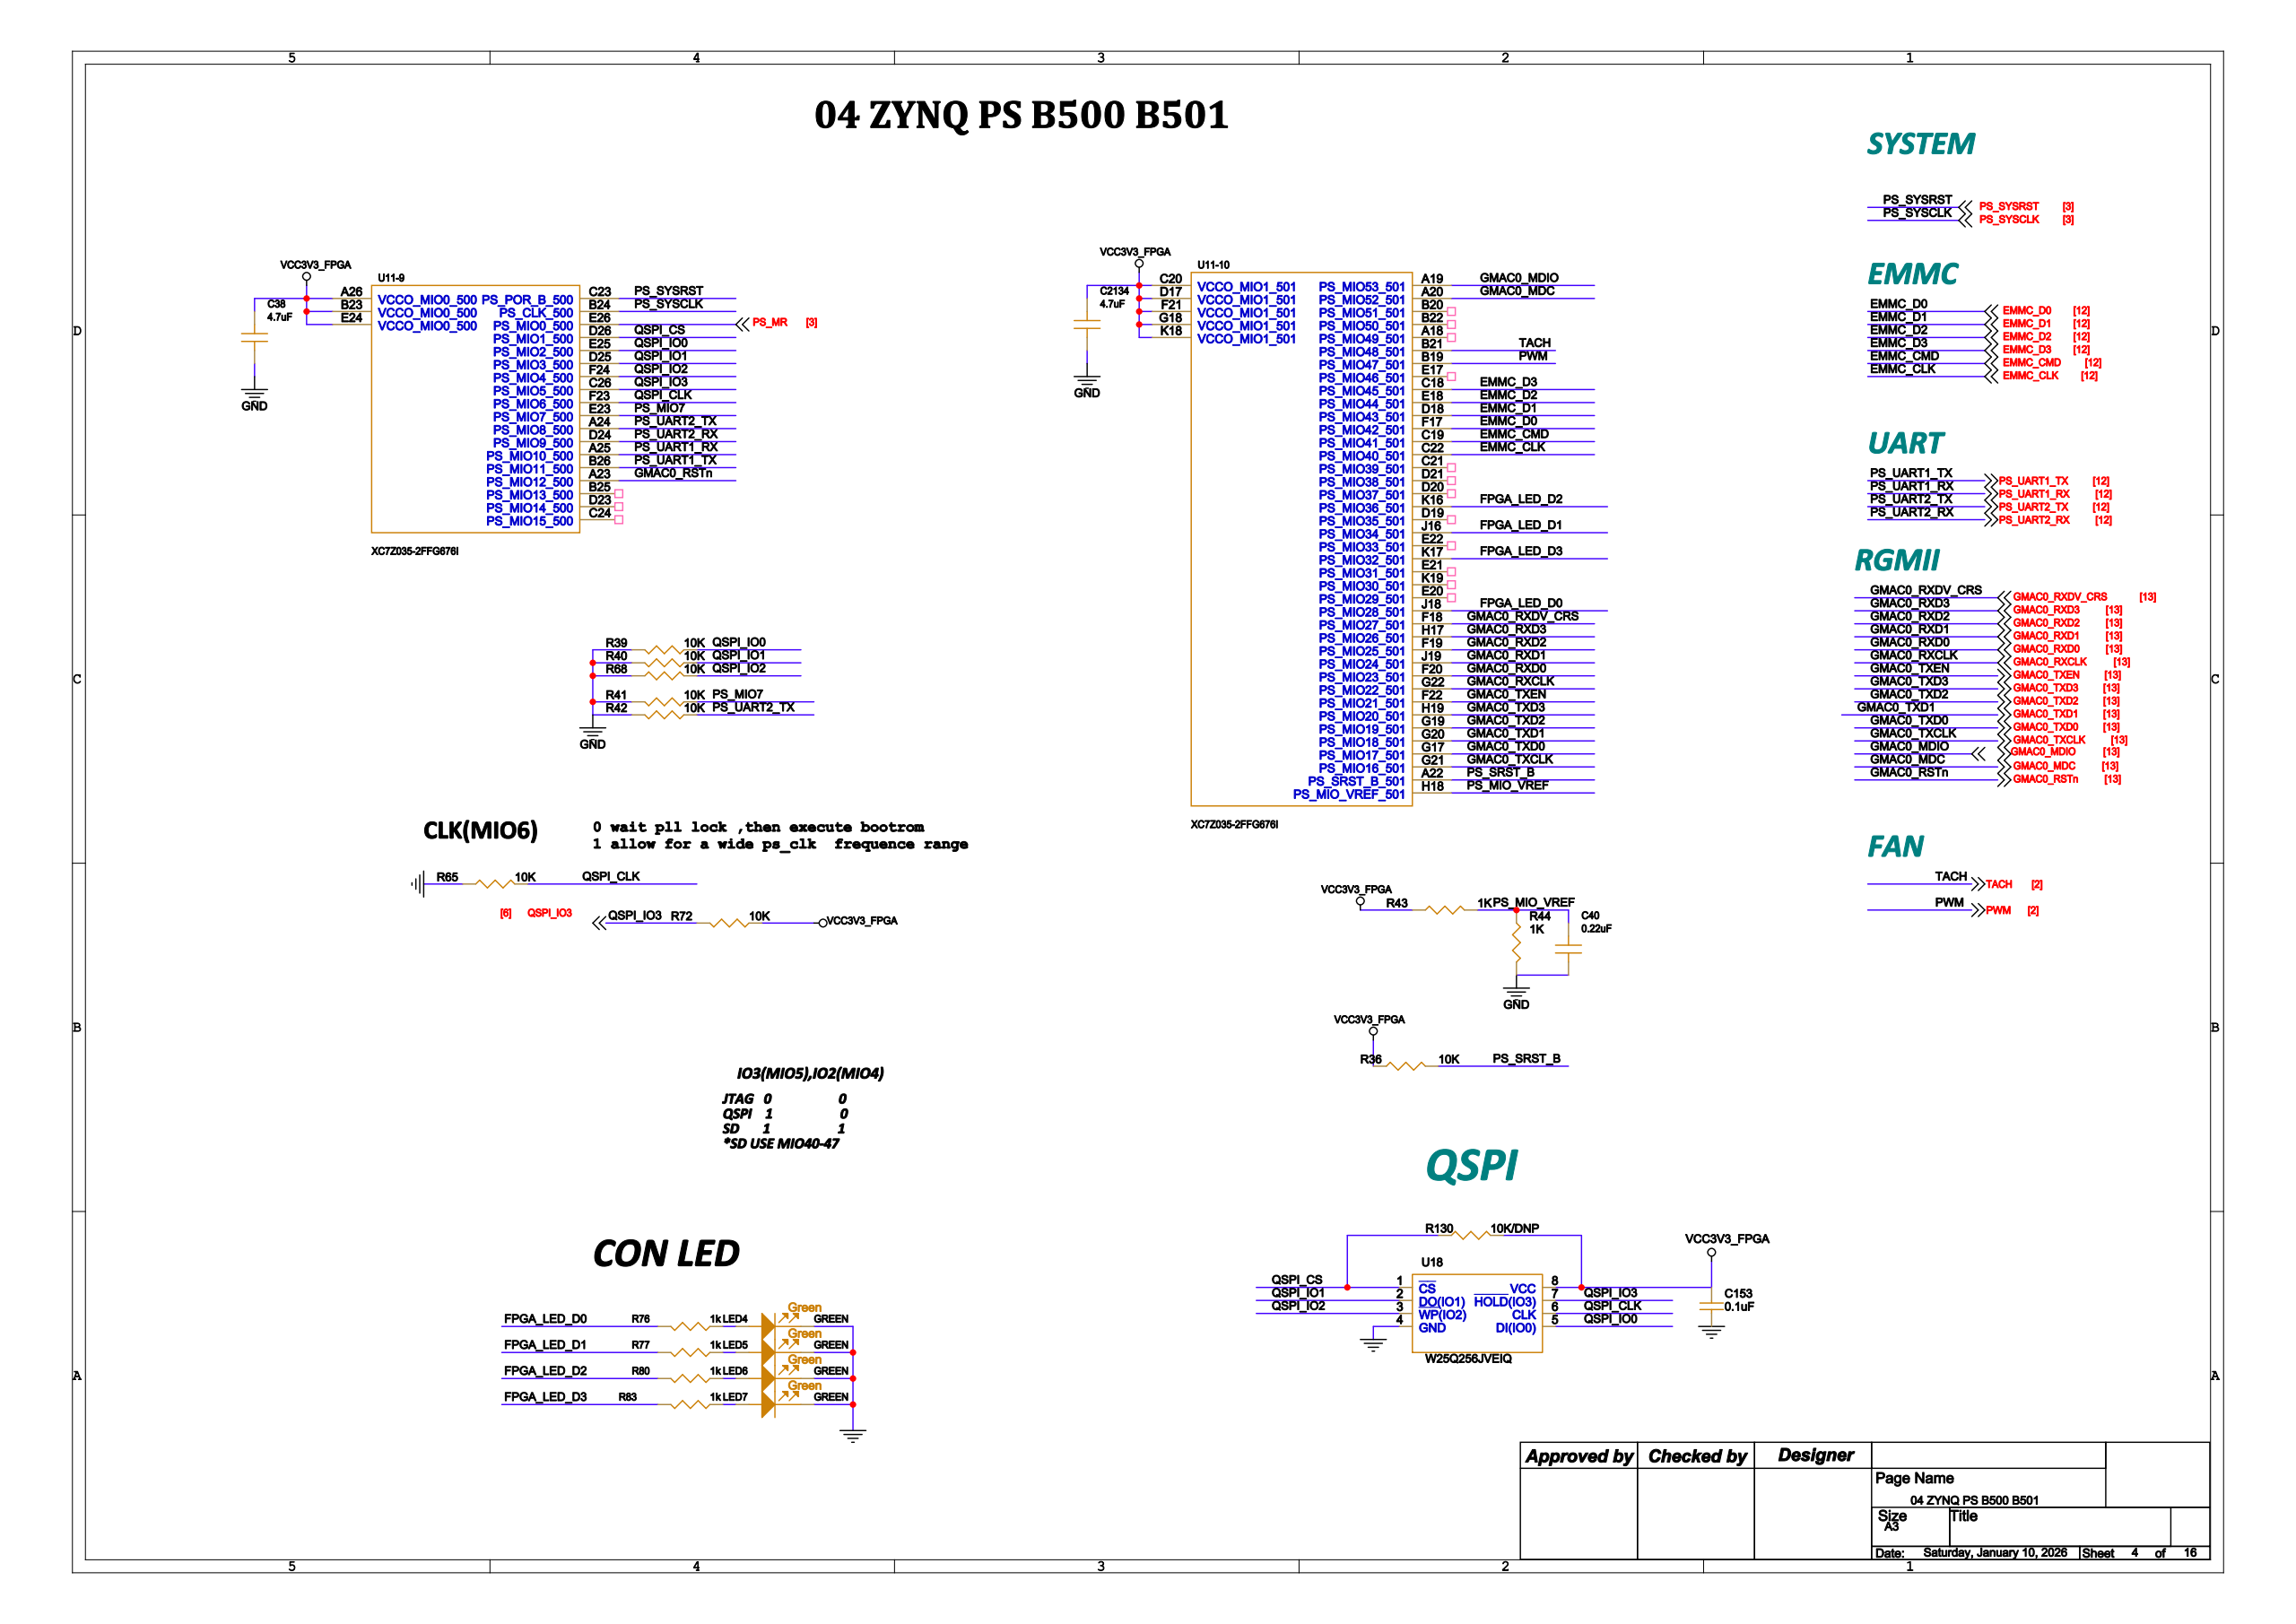Circuit board | Cadence Allegro | 442 parts | 326 nets | one sheet of the schematic
Parts on this sheet (reference | value | footprint):
C38 | 4.7uF | C0402_D
C40 | 0.22uF | C0201
C153 | 0.1uF | C0201
C2134 | 4.7uF | C0402_D
LED4 | GREEN | D0402
LED5 | GREEN | D0402
LED6 | GREEN | D0402
LED7 | GREEN | D0402
R36 | 10K | R0201
R39 | 10K | R0201
R40 | 10K | R0201
R41 | 10K | R0201
R42 | 10K | R0201
R43 | 1K | R0201
R44 | 1K | R0201
R65 | 10K | R0201
R68 | 10K | R0201
R72 | 10K | R0201
R76 | 1K | R0201
R77 | 1K | R0201
R80 | 1K | R0201
R83 | 1K | R0201
R130 | 10K/DNP | R0201
U18 | W25Q256JVEIQ | SO8-25X75-200
Nets of these parts (net: part-pin ...):
GND: C38-2 C40-2 C153-2 C2134-2 LED4-2 LED5-2 LED6-2 LED7-2 R39-2 R40-2 R41-2 R42-2 R44-2 R65-2 R68-2 U18-4
PS_UART2_TX: R42-1
VCC3V3_FPGA: C38-1 C153-1 C2134-1 R36-2 R43-1 R72-2 R130-1 U18-8
N49950527: LED4-1 R76-2
N49950552: LED5-1 R77-2
N49950577: LED6-1 R80-2
N49950594: LED7-1 R83-2
QSPI_IO3: R72-1 U18-7
PS_MIO_VREF: C40-1 R43-2 R44-1
QSPI_CS: R130-2 U18-1
FPGA_LED_D0: R76-1
FPGA_LED_D1: R77-1
FPGA_LED_D2: R80-1
FPGA_LED_D3: R83-1
PS_SRST_B: R36-1
QSPI_IO0: R39-1 U18-5
QSPI_IO1: R40-1 U18-2
PS_MIO7: R41-1
QSPI_CLK: R65-1 U18-6
QSPI_IO2: R68-1 U18-3